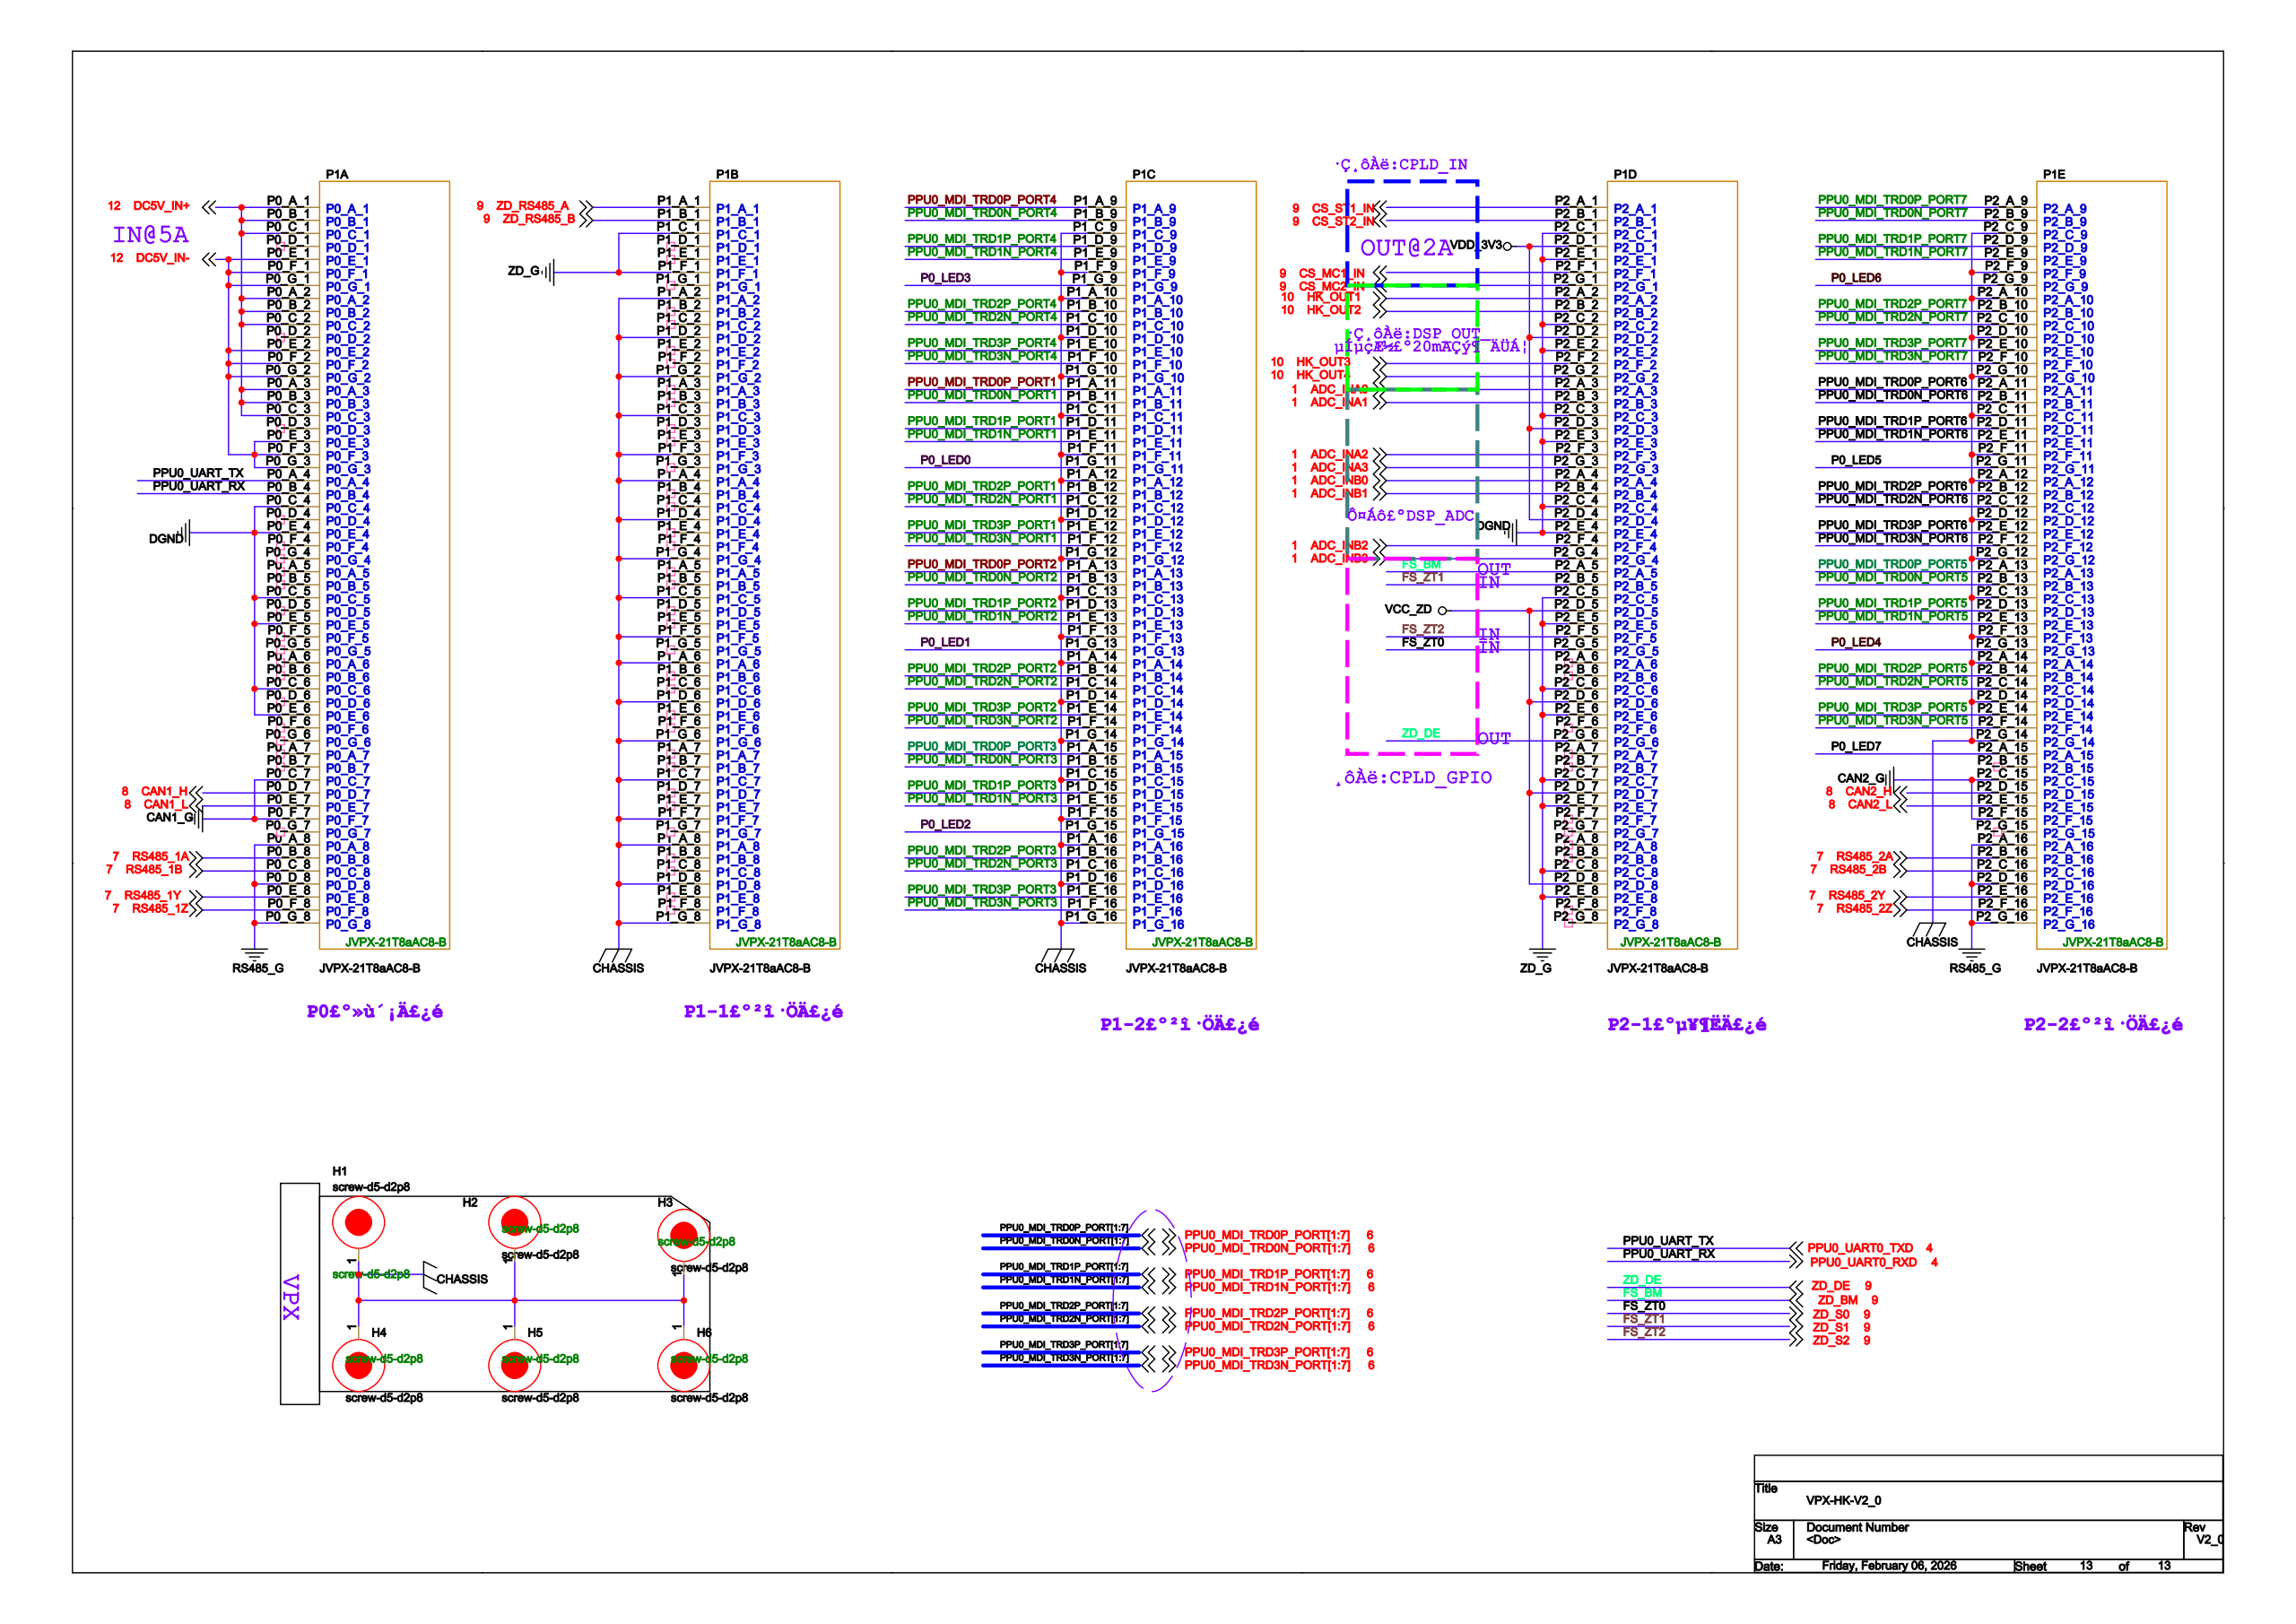Circuit board | Cadence Allegro | 598 parts | 541 nets | one sheet of the schematic
Parts on this sheet (reference | value | footprint):
H1 | screw-d5-d2p8 | SCREW-D5-D2P8
H2 | screw-d5-d2p8 | SCREW-D5-D2P8
H3 | screw-d5-d2p8 | SCREW-D5-D2P8
H4 | screw-d5-d2p8 | SCREW-D5-D2P8
H5 | screw-d5-d2p8 | SCREW-D5-D2P8
H6 | screw-d5-d2p8 | SCREW-D5-D2P8
P1 | JVPX-21T8aAC8-B | JVPX-21T8AAC8-B
Nets of these parts (net: part-pin ...):
DGND: P1-P0_C_4 P1-P0_C_5 P1-P0_C_6 P1-P0_E_4 P1-P0_E_5 P1-P0_E_6 P1-P2_C_1 P1-P2_C_2 P1-P2_C_3 P1-P2_C_4 P1-P2_E_1 P1-P2_E_2 P1-P2_E_3 P1-P2_E_4
DC5V_IN+: P1-P0_A_1 P1-P0_A_2 P1-P0_A_3 P1-P0_B_1 P1-P0_B_2 P1-P0_B_3 P1-P0_C_1 P1-P0_C_2 P1-P0_C_3
CHASSIS: H1-1 H2-1 H3-1 H4-1 H5-1 H6-1 P1-P1_A_2 P1-P1_A_4 P1-P1_A_6 P1-P1_A_8 P1-P1_A_10 P1-P1_A_12 P1-P1_A_14 P1-P1_A_16 P1-P1_C_3 P1-P1_C_5 P1-P1_C_7 P1-P1_C_9 P1-P1_C_11 P1-P1_C_13 P1-P1_C_15 P1-P1_D_2 P1-P1_D_4 P1-P1_D_6 P1-P1_D_8 P1-P1_D_10 P1-P1_D_12 P1-P1_D_14 P1-P1_D_16 P1-P1_F_3 P1-P1_F_5 P1-P1_F_7 P1-P1_F_9 P1-P1_F_11 P1-P1_F_13 P1-P1_F_15 P1-P1_G_2 P1-P1_G_4 P1-P1_G_6 P1-P1_G_8 P1-P1_G_10 P1-P1_G_12 P1-P1_G_14 P1-P1_G_16 P1-P2_A_10 P1-P2_A_12 P1-P2_A_14 P1-P2_C_9 P1-P2_C_11 P1-P2_C_13 P1-P2_D_10 P1-P2_D_12 P1-P2_D_14 P1-P2_F_9 P1-P2_F_11 P1-P2_F_13 P1-P2_G_10 P1-P2_G_12 P1-P2_G_14
CS_MC2_IN: P1-P2_G_1
CS_MC1_IN: P1-P2_F_1
CS_ST2_IN: P1-P2_B_1
CS_ST1_IN: P1-P2_A_1
ZD_RS485_A: P1-P1_A_1
ZD_RS485_B: P1-P1_B_1
ZD_G: P1-P1_C_1 P1-P1_F_1 P1-P2_C_5 P1-P2_C_6 P1-P2_C_7 P1-P2_C_8 P1-P2_E_5 P1-P2_E_6 P1-P2_E_7 P1-P2_E_8
VDD_3V3: P1-P2_D_1 P1-P2_D_2 P1-P2_D_3 P1-P2_D_4
VCC_ZD: P1-P2_D_5 P1-P2_D_6 P1-P2_D_7 P1-P2_D_8
RS485_1Y: P1-P0_E_8
RS485_1Z: P1-P0_F_8
RS485_G: P1-P0_A_8 P1-P0_D_8 P1-P0_G_8 P1-P2_A_16 P1-P2_D_16 P1-P2_G_16
RS485_2Z: P1-P2_F_16
RS485_2Y: P1-P2_E_16
CAN1_G: P1-P0_C_7 P1-P0_F_7
CAN2_G: P1-P2_C_15 P1-P2_F_15
PPU0_UART0_TXD: P1-P0_A_4
PPU0_UART0_RXD: P1-P0_B_4
RS485_1A: P1-P0_B_8
RS485_1B: P1-P0_C_8
CAN1_H: P1-P0_D_7
CAN1_L: P1-P0_E_7
PPU0_MDI_TRD0P_PORT1: P1-P1_A_11
PPU0_MDI_TRD0P_PORT2: P1-P1_A_13
PPU0_MDI_TRD0P_PORT3: P1-P1_A_15
PPU0_MDI_TRD0P_PORT4: P1-P1_A_9
PPU0_MDI_TRD2P_PORT4: P1-P1_B_10
PPU0_MDI_TRD0N_PORT1: P1-P1_B_11
PPU0_MDI_TRD2P_PORT1: P1-P1_B_12
PPU0_MDI_TRD0N_PORT2: P1-P1_B_13
PPU0_MDI_TRD2P_PORT2: P1-P1_B_14
PPU0_MDI_TRD0N_PORT3: P1-P1_B_15
PPU0_MDI_TRD2P_PORT3: P1-P1_B_16
PPU0_MDI_TRD0N_PORT4: P1-P1_B_9
PPU0_MDI_TRD2N_PORT4: P1-P1_C_10
PPU0_MDI_TRD2N_PORT1: P1-P1_C_12
PPU0_MDI_TRD2N_PORT2: P1-P1_C_14
PPU0_MDI_TRD2N_PORT3: P1-P1_C_16
PPU0_MDI_TRD1P_PORT1: P1-P1_D_11
PPU0_MDI_TRD1P_PORT2: P1-P1_D_13
PPU0_MDI_TRD1P_PORT3: P1-P1_D_15
PPU0_MDI_TRD1P_PORT4: P1-P1_D_9
PPU0_MDI_TRD3P_PORT4: P1-P1_E_10
PPU0_MDI_TRD1N_PORT1: P1-P1_E_11
PPU0_MDI_TRD3P_PORT1: P1-P1_E_12
PPU0_MDI_TRD1N_PORT2: P1-P1_E_13
PPU0_MDI_TRD3P_PORT2: P1-P1_E_14
PPU0_MDI_TRD1N_PORT3: P1-P1_E_15
PPU0_MDI_TRD3P_PORT3: P1-P1_E_16
PPU0_MDI_TRD1N_PORT4: P1-P1_E_9
PPU0_MDI_TRD3N_PORT4: P1-P1_F_10
PPU0_MDI_TRD3N_PORT1: P1-P1_F_12
PPU0_MDI_TRD3N_PORT2: P1-P1_F_14
PPU0_MDI_TRD3N_PORT3: P1-P1_F_16
P0_LED0: P1-P1_G_11
P0_LED1: P1-P1_G_13
P0_LED2: P1-P1_G_15
P0_LED3: P1-P1_G_9
HK_OUT1: P1-P2_A_2
ADC_INA0: P1-P2_A_3
ADC_INB0: P1-P2_A_4
ZD_BM: P1-P2_A_5
HK_OUT2: P1-P2_B_2
ADC_INA1: P1-P2_B_3
ADC_INB1: P1-P2_B_4
ZD_S1: P1-P2_B_5
HK_OUT3: P1-P2_F_2
ADC_INA2: P1-P2_F_3
ADC_INB2: P1-P2_F_4
ZD_S2: P1-P2_F_5
HK_OUT4: P1-P2_G_2
ADC_INA3: P1-P2_G_3
ADC_INB3: P1-P2_G_4
ZD_S0: P1-P2_G_5
ZD_DE: P1-P2_G_6
PPU0_MDI_TRD0P_PORT6: P1-P2_A_11
PPU0_MDI_TRD0P_PORT5: P1-P2_A_13
P0_LED7: P1-P2_A_15
PPU0_MDI_TRD0P_PORT7: P1-P2_A_9
PPU0_MDI_TRD2P_PORT7: P1-P2_B_10
PPU0_MDI_TRD0N_PORT6: P1-P2_B_11
PPU0_MDI_TRD2P_PORT6: P1-P2_B_12
PPU0_MDI_TRD0N_PORT5: P1-P2_B_13
PPU0_MDI_TRD2P_PORT5: P1-P2_B_14
RS485_2A: P1-P2_B_16
PPU0_MDI_TRD0N_PORT7: P1-P2_B_9
PPU0_MDI_TRD2N_PORT7: P1-P2_C_10
PPU0_MDI_TRD2N_PORT6: P1-P2_C_12
PPU0_MDI_TRD2N_PORT5: P1-P2_C_14
RS485_2B: P1-P2_C_16
PPU0_MDI_TRD1P_PORT6: P1-P2_D_11
PPU0_MDI_TRD1P_PORT5: P1-P2_D_13
CAN2_H: P1-P2_D_15
PPU0_MDI_TRD1P_PORT7: P1-P2_D_9
PPU0_MDI_TRD3P_PORT7: P1-P2_E_10
PPU0_MDI_TRD1N_PORT6: P1-P2_E_11
PPU0_MDI_TRD3P_PORT6: P1-P2_E_12
PPU0_MDI_TRD1N_PORT5: P1-P2_E_13
PPU0_MDI_TRD3P_PORT5: P1-P2_E_14
CAN2_L: P1-P2_E_15
PPU0_MDI_TRD1N_PORT7: P1-P2_E_9
PPU0_MDI_TRD3N_PORT7: P1-P2_F_10
PPU0_MDI_TRD3N_PORT6: P1-P2_F_12
PPU0_MDI_TRD3N_PORT5: P1-P2_F_14
P0_LED5: P1-P2_G_11
P0_LED4: P1-P2_G_13
P0_LED6: P1-P2_G_9